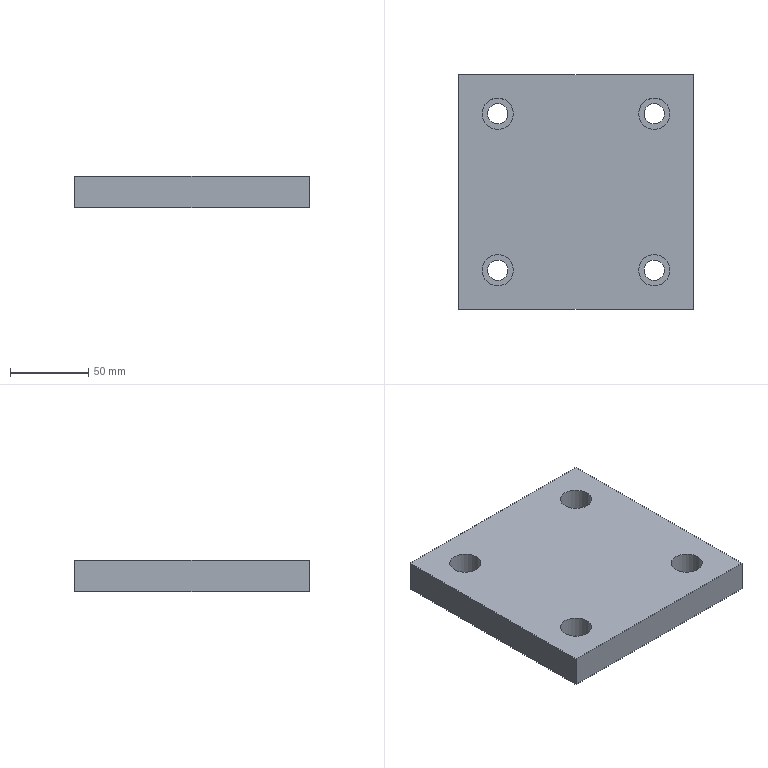Part | NX | features solid 2 | 1 solid | 18 faces | box 150 x 150 x 20 mm | volume 429222 mm3 | plane 10 | cylinder 8 | commonest cylinder face diameters 13 x4 20 x4
STEP:
#1=CARTESIAN_POINT('',(335.,1005.,-255.));
#2=VERTEX_POINT('',#1);
#3=CARTESIAN_POINT('',(335.,855.,-255.));
#4=VERTEX_POINT('',#3);
#5=CARTESIAN_POINT('',(335.,1032.5,-255.));
#6=DIRECTION('',(0.,1.,0.));
#7=VECTOR('',#6,1000.);
#8=LINE('',#5,#7);
#9=EDGE_CURVE('',#2,#4,#8,.F.);
#10=ORIENTED_EDGE('',*,*,#9,.T.);
#11=CARTESIAN_POINT('',(185.,855.,-255.));
#12=VERTEX_POINT('',#11);
#13=CARTESIAN_POINT('',(222.674,855.,-255.));
#14=DIRECTION('',(-1.,0.,0.));
#15=VECTOR('',#14,1000.);
#16=LINE('',#13,#15);
#17=EDGE_CURVE('',#12,#4,#16,.F.);
#18=ORIENTED_EDGE('',*,*,#17,.F.);
#19=CARTESIAN_POINT('',(185.,1005.,-255.));
#20=VERTEX_POINT('',#19);
#21=CARTESIAN_POINT('',(185.,1032.5,-255.));
#22=DIRECTION('',(0.,-1.,0.));
#23=VECTOR('',#22,1000.);
#24=LINE('',#21,#23);
#25=EDGE_CURVE('',#12,#20,#24,.F.);
#26=ORIENTED_EDGE('',*,*,#25,.T.);
#27=CARTESIAN_POINT('',(222.674,1005.,-255.));
#28=DIRECTION('',(-1.,0.,0.));
#29=VECTOR('',#28,1000.);
#30=LINE('',#27,#29);
#31=EDGE_CURVE('',#20,#2,#30,.F.);
#32=ORIENTED_EDGE('',*,*,#31,.T.);
#33=EDGE_LOOP('',(#10,#18,#26,#32));
#34=FACE_BOUND('',#33,.T.);
#35=CARTESIAN_POINT('',(210.,986.5,-255.));
#36=VERTEX_POINT('',#35);
#37=CARTESIAN_POINT('',(210.,980.,-255.));
#38=DIRECTION('',(0.,0.,-1.));
#39=DIRECTION('',(0.,1.,0.));
#40=AXIS2_PLACEMENT_3D('',#37,#38,#39);
#41=CIRCLE('',#40,6.5);
#42=EDGE_CURVE('',#36,#36,#41,.T.);
#43=ORIENTED_EDGE('',*,*,#42,.F.);
#44=EDGE_LOOP('',(#43));
#45=FACE_BOUND('',#44,.T.);
#46=CARTESIAN_POINT('',(310.,986.5,-255.));
#47=VERTEX_POINT('',#46);
#48=CARTESIAN_POINT('',(310.,980.,-255.));
#49=DIRECTION('',(0.,0.,-1.));
#50=DIRECTION('',(0.,1.,0.));
#51=AXIS2_PLACEMENT_3D('',#48,#49,#50);
#52=CIRCLE('',#51,6.5);
#53=EDGE_CURVE('',#47,#47,#52,.T.);
#54=ORIENTED_EDGE('',*,*,#53,.F.);
#55=EDGE_LOOP('',(#54));
#56=FACE_BOUND('',#55,.T.);
#57=CARTESIAN_POINT('',(210.,886.5,-255.));
#58=VERTEX_POINT('',#57);
#59=CARTESIAN_POINT('',(210.,880.,-255.));
#60=DIRECTION('',(0.,0.,-1.));
#61=DIRECTION('',(0.,1.,0.));
#62=AXIS2_PLACEMENT_3D('',#59,#60,#61);
#63=CIRCLE('',#62,6.5);
#64=EDGE_CURVE('',#58,#58,#63,.T.);
#65=ORIENTED_EDGE('',*,*,#64,.F.);
#66=EDGE_LOOP('',(#65));
#67=FACE_BOUND('',#66,.T.);
#68=CARTESIAN_POINT('',(310.,886.5,-255.));
#69=VERTEX_POINT('',#68);
#70=CARTESIAN_POINT('',(310.,880.,-255.));
#71=DIRECTION('',(0.,0.,-1.));
#72=DIRECTION('',(0.,1.,0.));
#73=AXIS2_PLACEMENT_3D('',#70,#71,#72);
#74=CIRCLE('',#73,6.5);
#75=EDGE_CURVE('',#69,#69,#74,.T.);
#76=ORIENTED_EDGE('',*,*,#75,.F.);
#77=EDGE_LOOP('',(#76));
#78=FACE_BOUND('',#77,.T.);
#79=CARTESIAN_POINT('',(222.674,1032.5,-255.));
#80=DIRECTION('',(0.,0.,1.));
#81=DIRECTION('',(1.,0.,0.));
#82=AXIS2_PLACEMENT_3D('',#79,#80,#81);
#83=PLANE('',#82);
#84=ADVANCED_FACE('',(#34,#45,#56,#67,#78),#83,.F.);
#85=CARTESIAN_POINT('',(185.,1005.,-235.));
#86=VERTEX_POINT('',#85);
#87=CARTESIAN_POINT('',(335.,1005.,-235.));
#88=VERTEX_POINT('',#87);
#89=CARTESIAN_POINT('',(222.674,1005.,-235.));
#90=DIRECTION('',(-1.,0.,0.));
#91=VECTOR('',#90,1000.);
#92=LINE('',#89,#91);
#93=EDGE_CURVE('',#86,#88,#92,.F.);
#94=ORIENTED_EDGE('',*,*,#93,.F.);
#95=CARTESIAN_POINT('',(185.,855.,-235.));
#96=VERTEX_POINT('',#95);
#97=CARTESIAN_POINT('',(185.,1032.5,-235.));
#98=DIRECTION('',(0.,-1.,0.));
#99=VECTOR('',#98,1000.);
#100=LINE('',#97,#99);
#101=EDGE_CURVE('',#96,#86,#100,.F.);
#102=ORIENTED_EDGE('',*,*,#101,.F.);
#103=CARTESIAN_POINT('',(335.,855.,-235.));
#104=VERTEX_POINT('',#103);
#105=CARTESIAN_POINT('',(222.674,855.,-235.));
#106=DIRECTION('',(-1.,0.,0.));
#107=VECTOR('',#106,1000.);
#108=LINE('',#105,#107);
#109=EDGE_CURVE('',#96,#104,#108,.F.);
#110=ORIENTED_EDGE('',*,*,#109,.T.);
#111=CARTESIAN_POINT('',(335.,1032.5,-235.));
#112=DIRECTION('',(0.,1.,0.));
#113=VECTOR('',#112,1000.);
#114=LINE('',#111,#113);
#115=EDGE_CURVE('',#88,#104,#114,.F.);
#116=ORIENTED_EDGE('',*,*,#115,.F.);
#117=EDGE_LOOP('',(#94,#102,#110,#116));
#118=FACE_BOUND('',#117,.T.);
#119=CARTESIAN_POINT('',(210.,990.,-235.));
#120=VERTEX_POINT('',#119);
#121=CARTESIAN_POINT('',(210.,980.,-235.));
#122=DIRECTION('',(0.,0.,-1.));
#123=DIRECTION('',(0.,1.,0.));
#124=AXIS2_PLACEMENT_3D('',#121,#122,#123);
#125=CIRCLE('',#124,10.);
#126=EDGE_CURVE('',#120,#120,#125,.T.);
#127=ORIENTED_EDGE('',*,*,#126,.T.);
#128=EDGE_LOOP('',(#127));
#129=FACE_BOUND('',#128,.T.);
#130=CARTESIAN_POINT('',(310.,990.,-235.));
#131=VERTEX_POINT('',#130);
#132=CARTESIAN_POINT('',(310.,980.,-235.));
#133=DIRECTION('',(0.,0.,-1.));
#134=DIRECTION('',(0.,1.,0.));
#135=AXIS2_PLACEMENT_3D('',#132,#133,#134);
#136=CIRCLE('',#135,10.);
#137=EDGE_CURVE('',#131,#131,#136,.T.);
#138=ORIENTED_EDGE('',*,*,#137,.T.);
#139=EDGE_LOOP('',(#138));
#140=FACE_BOUND('',#139,.T.);
#141=CARTESIAN_POINT('',(210.,890.,-235.));
#142=VERTEX_POINT('',#141);
#143=CARTESIAN_POINT('',(210.,880.,-235.));
#144=DIRECTION('',(0.,0.,-1.));
#145=DIRECTION('',(0.,1.,0.));
#146=AXIS2_PLACEMENT_3D('',#143,#144,#145);
#147=CIRCLE('',#146,10.);
#148=EDGE_CURVE('',#142,#142,#147,.T.);
#149=ORIENTED_EDGE('',*,*,#148,.T.);
#150=EDGE_LOOP('',(#149));
#151=FACE_BOUND('',#150,.T.);
#152=CARTESIAN_POINT('',(310.,890.,-235.));
#153=VERTEX_POINT('',#152);
#154=CARTESIAN_POINT('',(310.,880.,-235.));
#155=DIRECTION('',(0.,0.,-1.));
#156=DIRECTION('',(0.,1.,0.));
#157=AXIS2_PLACEMENT_3D('',#154,#155,#156);
#158=CIRCLE('',#157,10.);
#159=EDGE_CURVE('',#153,#153,#158,.T.);
#160=ORIENTED_EDGE('',*,*,#159,.T.);
#161=EDGE_LOOP('',(#160));
#162=FACE_BOUND('',#161,.T.);
#163=CARTESIAN_POINT('',(222.674,1032.5,-235.));
#164=DIRECTION('',(0.,0.,1.));
#165=DIRECTION('',(1.,0.,0.));
#166=AXIS2_PLACEMENT_3D('',#163,#164,#165);
#167=PLANE('',#166);
#168=ADVANCED_FACE('',(#118,#129,#140,#151,#162),#167,.T.);
#169=CARTESIAN_POINT('',(185.,1005.,-255.));
#170=DIRECTION('',(0.,0.,1.));
#171=VECTOR('',#170,1000.);
#172=LINE('',#169,#171);
#173=EDGE_CURVE('',#20,#86,#172,.T.);
#174=ORIENTED_EDGE('',*,*,#173,.F.);
#175=ORIENTED_EDGE('',*,*,#25,.F.);
#176=CARTESIAN_POINT('',(185.,855.,-255.));
#177=DIRECTION('',(0.,0.,1.));
#178=VECTOR('',#177,1000.);
#179=LINE('',#176,#178);
#180=EDGE_CURVE('',#12,#96,#179,.T.);
#181=ORIENTED_EDGE('',*,*,#180,.T.);
#182=ORIENTED_EDGE('',*,*,#101,.T.);
#183=EDGE_LOOP('',(#174,#175,#181,#182));
#184=FACE_BOUND('',#183,.T.);
#185=CARTESIAN_POINT('',(185.,1032.5,-255.));
#186=DIRECTION('',(1.,0.,0.));
#187=DIRECTION('',(0.,0.,1.));
#188=AXIS2_PLACEMENT_3D('',#185,#186,#187);
#189=PLANE('',#188);
#190=ADVANCED_FACE('',(#184),#189,.F.);
#191=ORIENTED_EDGE('',*,*,#115,.T.);
#192=CARTESIAN_POINT('',(335.,855.,-255.));
#193=DIRECTION('',(0.,0.,1.));
#194=VECTOR('',#193,1000.);
#195=LINE('',#192,#194);
#196=EDGE_CURVE('',#4,#104,#195,.T.);
#197=ORIENTED_EDGE('',*,*,#196,.F.);
#198=ORIENTED_EDGE('',*,*,#9,.F.);
#199=CARTESIAN_POINT('',(335.,1005.,-255.));
#200=DIRECTION('',(0.,0.,1.));
#201=VECTOR('',#200,1000.);
#202=LINE('',#199,#201);
#203=EDGE_CURVE('',#2,#88,#202,.T.);
#204=ORIENTED_EDGE('',*,*,#203,.T.);
#205=EDGE_LOOP('',(#191,#197,#198,#204));
#206=FACE_BOUND('',#205,.T.);
#207=CARTESIAN_POINT('',(335.,1007.5,-255.));
#208=DIRECTION('',(1.,0.,0.));
#209=DIRECTION('',(0.,0.,1.));
#210=AXIS2_PLACEMENT_3D('',#207,#208,#209);
#211=PLANE('',#210);
#212=ADVANCED_FACE('',(#206),#211,.T.);
#213=ORIENTED_EDGE('',*,*,#17,.T.);
#214=ORIENTED_EDGE('',*,*,#196,.T.);
#215=ORIENTED_EDGE('',*,*,#109,.F.);
#216=ORIENTED_EDGE('',*,*,#180,.F.);
#217=EDGE_LOOP('',(#213,#214,#215,#216));
#218=FACE_BOUND('',#217,.T.);
#219=CARTESIAN_POINT('',(222.674,855.,-255.));
#220=DIRECTION('',(0.,-1.,0.));
#221=DIRECTION('',(0.,0.,-1.));
#222=AXIS2_PLACEMENT_3D('',#219,#220,#221);
#223=PLANE('',#222);
#224=ADVANCED_FACE('',(#218),#223,.T.);
#225=ORIENTED_EDGE('',*,*,#75,.T.);
#226=EDGE_LOOP('',(#225));
#227=FACE_BOUND('',#226,.T.);
#228=CARTESIAN_POINT('',(310.,886.5,-249.));
#229=VERTEX_POINT('',#228);
#230=CARTESIAN_POINT('',(310.,880.,-249.));
#231=DIRECTION('',(0.,0.,-1.));
#232=DIRECTION('',(0.,1.,0.));
#233=AXIS2_PLACEMENT_3D('',#230,#231,#232);
#234=CIRCLE('',#233,6.5);
#235=EDGE_CURVE('',#229,#229,#234,.T.);
#236=ORIENTED_EDGE('',*,*,#235,.F.);
#237=EDGE_LOOP('',(#236));
#238=FACE_BOUND('',#237,.T.);
#239=CARTESIAN_POINT('',(310.,880.,-255.));
#240=DIRECTION('',(0.,0.,-1.));
#241=DIRECTION('',(0.,1.,0.));
#242=AXIS2_PLACEMENT_3D('',#239,#240,#241);
#243=CYLINDRICAL_SURFACE('',#242,6.5);
#244=ADVANCED_FACE('',(#227,#238),#243,.F.);
#245=ORIENTED_EDGE('',*,*,#235,.T.);
#246=EDGE_LOOP('',(#245));
#247=FACE_BOUND('',#246,.T.);
#248=CARTESIAN_POINT('',(310.,890.,-249.));
#249=VERTEX_POINT('',#248);
#250=CARTESIAN_POINT('',(310.,880.,-249.));
#251=DIRECTION('',(0.,0.,-1.));
#252=DIRECTION('',(0.,1.,0.));
#253=AXIS2_PLACEMENT_3D('',#250,#251,#252);
#254=CIRCLE('',#253,10.);
#255=EDGE_CURVE('',#249,#249,#254,.T.);
#256=ORIENTED_EDGE('',*,*,#255,.F.);
#257=EDGE_LOOP('',(#256));
#258=FACE_BOUND('',#257,.T.);
#259=CARTESIAN_POINT('',(310.,880.,-249.));
#260=DIRECTION('',(0.,0.,-1.));
#261=DIRECTION('',(0.,1.,0.));
#262=AXIS2_PLACEMENT_3D('',#259,#260,#261);
#263=PLANE('',#262);
#264=ADVANCED_FACE('',(#247,#258),#263,.F.);
#265=ORIENTED_EDGE('',*,*,#255,.T.);
#266=EDGE_LOOP('',(#265));
#267=FACE_BOUND('',#266,.T.);
#268=ORIENTED_EDGE('',*,*,#159,.F.);
#269=EDGE_LOOP('',(#268));
#270=FACE_BOUND('',#269,.T.);
#271=CARTESIAN_POINT('',(310.,880.,-235.));
#272=DIRECTION('',(0.,0.,-1.));
#273=DIRECTION('',(0.,1.,0.));
#274=AXIS2_PLACEMENT_3D('',#271,#272,#273);
#275=CYLINDRICAL_SURFACE('',#274,10.);
#276=ADVANCED_FACE('',(#267,#270),#275,.F.);
#277=ORIENTED_EDGE('',*,*,#64,.T.);
#278=EDGE_LOOP('',(#277));
#279=FACE_BOUND('',#278,.T.);
#280=CARTESIAN_POINT('',(210.,886.5,-249.));
#281=VERTEX_POINT('',#280);
#282=CARTESIAN_POINT('',(210.,880.,-249.));
#283=DIRECTION('',(0.,0.,-1.));
#284=DIRECTION('',(0.,1.,0.));
#285=AXIS2_PLACEMENT_3D('',#282,#283,#284);
#286=CIRCLE('',#285,6.5);
#287=EDGE_CURVE('',#281,#281,#286,.T.);
#288=ORIENTED_EDGE('',*,*,#287,.F.);
#289=EDGE_LOOP('',(#288));
#290=FACE_BOUND('',#289,.T.);
#291=CARTESIAN_POINT('',(210.,880.,-255.));
#292=DIRECTION('',(0.,0.,-1.));
#293=DIRECTION('',(0.,1.,0.));
#294=AXIS2_PLACEMENT_3D('',#291,#292,#293);
#295=CYLINDRICAL_SURFACE('',#294,6.5);
#296=ADVANCED_FACE('',(#279,#290),#295,.F.);
#297=ORIENTED_EDGE('',*,*,#287,.T.);
#298=EDGE_LOOP('',(#297));
#299=FACE_BOUND('',#298,.T.);
#300=CARTESIAN_POINT('',(210.,890.,-249.));
#301=VERTEX_POINT('',#300);
#302=CARTESIAN_POINT('',(210.,880.,-249.));
#303=DIRECTION('',(0.,0.,-1.));
#304=DIRECTION('',(0.,1.,0.));
#305=AXIS2_PLACEMENT_3D('',#302,#303,#304);
#306=CIRCLE('',#305,10.);
#307=EDGE_CURVE('',#301,#301,#306,.T.);
#308=ORIENTED_EDGE('',*,*,#307,.F.);
#309=EDGE_LOOP('',(#308));
#310=FACE_BOUND('',#309,.T.);
#311=CARTESIAN_POINT('',(210.,880.,-249.));
#312=DIRECTION('',(0.,0.,-1.));
#313=DIRECTION('',(0.,1.,0.));
#314=AXIS2_PLACEMENT_3D('',#311,#312,#313);
#315=PLANE('',#314);
#316=ADVANCED_FACE('',(#299,#310),#315,.F.);
#317=ORIENTED_EDGE('',*,*,#307,.T.);
#318=EDGE_LOOP('',(#317));
#319=FACE_BOUND('',#318,.T.);
#320=ORIENTED_EDGE('',*,*,#148,.F.);
#321=EDGE_LOOP('',(#320));
#322=FACE_BOUND('',#321,.T.);
#323=CARTESIAN_POINT('',(210.,880.,-235.));
#324=DIRECTION('',(0.,0.,-1.));
#325=DIRECTION('',(0.,1.,0.));
#326=AXIS2_PLACEMENT_3D('',#323,#324,#325);
#327=CYLINDRICAL_SURFACE('',#326,10.);
#328=ADVANCED_FACE('',(#319,#322),#327,.F.);
#329=CARTESIAN_POINT('',(310.,986.5,-249.));
#330=VERTEX_POINT('',#329);
#331=CARTESIAN_POINT('',(310.,980.,-249.));
#332=DIRECTION('',(0.,0.,-1.));
#333=DIRECTION('',(0.,1.,0.));
#334=AXIS2_PLACEMENT_3D('',#331,#332,#333);
#335=CIRCLE('',#334,6.5);
#336=EDGE_CURVE('',#330,#330,#335,.T.);
#337=ORIENTED_EDGE('',*,*,#336,.T.);
#338=EDGE_LOOP('',(#337));
#339=FACE_BOUND('',#338,.T.);
#340=CARTESIAN_POINT('',(310.,990.,-249.));
#341=VERTEX_POINT('',#340);
#342=CARTESIAN_POINT('',(310.,980.,-249.));
#343=DIRECTION('',(0.,0.,-1.));
#344=DIRECTION('',(0.,1.,0.));
#345=AXIS2_PLACEMENT_3D('',#342,#343,#344);
#346=CIRCLE('',#345,10.);
#347=EDGE_CURVE('',#341,#341,#346,.T.);
#348=ORIENTED_EDGE('',*,*,#347,.F.);
#349=EDGE_LOOP('',(#348));
#350=FACE_BOUND('',#349,.T.);
#351=CARTESIAN_POINT('',(310.,980.,-249.));
#352=DIRECTION('',(0.,0.,-1.));
#353=DIRECTION('',(0.,1.,0.));
#354=AXIS2_PLACEMENT_3D('',#351,#352,#353);
#355=PLANE('',#354);
#356=ADVANCED_FACE('',(#339,#350),#355,.F.);
#357=CARTESIAN_POINT('',(210.,986.5,-249.));
#358=VERTEX_POINT('',#357);
#359=CARTESIAN_POINT('',(210.,980.,-249.));
#360=DIRECTION('',(0.,0.,-1.));
#361=DIRECTION('',(0.,1.,0.));
#362=AXIS2_PLACEMENT_3D('',#359,#360,#361);
#363=CIRCLE('',#362,6.5);
#364=EDGE_CURVE('',#358,#358,#363,.T.);
#365=ORIENTED_EDGE('',*,*,#364,.T.);
#366=EDGE_LOOP('',(#365));
#367=FACE_BOUND('',#366,.T.);
#368=CARTESIAN_POINT('',(210.,990.,-249.));
#369=VERTEX_POINT('',#368);
#370=CARTESIAN_POINT('',(210.,980.,-249.));
#371=DIRECTION('',(0.,0.,-1.));
#372=DIRECTION('',(0.,1.,0.));
#373=AXIS2_PLACEMENT_3D('',#370,#371,#372);
#374=CIRCLE('',#373,10.);
#375=EDGE_CURVE('',#369,#369,#374,.T.);
#376=ORIENTED_EDGE('',*,*,#375,.F.);
#377=EDGE_LOOP('',(#376));
#378=FACE_BOUND('',#377,.T.);
#379=CARTESIAN_POINT('',(210.,980.,-249.));
#380=DIRECTION('',(0.,0.,-1.));
#381=DIRECTION('',(0.,1.,0.));
#382=AXIS2_PLACEMENT_3D('',#379,#380,#381);
#383=PLANE('',#382);
#384=ADVANCED_FACE('',(#367,#378),#383,.F.);
#385=ORIENTED_EDGE('',*,*,#53,.T.);
#386=EDGE_LOOP('',(#385));
#387=FACE_BOUND('',#386,.T.);
#388=ORIENTED_EDGE('',*,*,#336,.F.);
#389=EDGE_LOOP('',(#388));
#390=FACE_BOUND('',#389,.T.);
#391=CARTESIAN_POINT('',(310.,980.,-255.));
#392=DIRECTION('',(0.,0.,-1.));
#393=DIRECTION('',(0.,1.,0.));
#394=AXIS2_PLACEMENT_3D('',#391,#392,#393);
#395=CYLINDRICAL_SURFACE('',#394,6.5);
#396=ADVANCED_FACE('',(#387,#390),#395,.F.);
#397=ORIENTED_EDGE('',*,*,#42,.T.);
#398=EDGE_LOOP('',(#397));
#399=FACE_BOUND('',#398,.T.);
#400=ORIENTED_EDGE('',*,*,#364,.F.);
#401=EDGE_LOOP('',(#400));
#402=FACE_BOUND('',#401,.T.);
#403=CARTESIAN_POINT('',(210.,980.,-255.));
#404=DIRECTION('',(0.,0.,-1.));
#405=DIRECTION('',(0.,1.,0.));
#406=AXIS2_PLACEMENT_3D('',#403,#404,#405);
#407=CYLINDRICAL_SURFACE('',#406,6.5);
#408=ADVANCED_FACE('',(#399,#402),#407,.F.);
#409=ORIENTED_EDGE('',*,*,#347,.T.);
#410=EDGE_LOOP('',(#409));
#411=FACE_BOUND('',#410,.T.);
#412=ORIENTED_EDGE('',*,*,#137,.F.);
#413=EDGE_LOOP('',(#412));
#414=FACE_BOUND('',#413,.T.);
#415=CARTESIAN_POINT('',(310.,980.,-235.));
#416=DIRECTION('',(0.,0.,-1.));
#417=DIRECTION('',(0.,1.,0.));
#418=AXIS2_PLACEMENT_3D('',#415,#416,#417);
#419=CYLINDRICAL_SURFACE('',#418,10.);
#420=ADVANCED_FACE('',(#411,#414),#419,.F.);
#421=ORIENTED_EDGE('',*,*,#375,.T.);
#422=EDGE_LOOP('',(#421));
#423=FACE_BOUND('',#422,.T.);
#424=ORIENTED_EDGE('',*,*,#126,.F.);
#425=EDGE_LOOP('',(#424));
#426=FACE_BOUND('',#425,.T.);
#427=CARTESIAN_POINT('',(210.,980.,-235.));
#428=DIRECTION('',(0.,0.,-1.));
#429=DIRECTION('',(0.,1.,0.));
#430=AXIS2_PLACEMENT_3D('',#427,#428,#429);
#431=CYLINDRICAL_SURFACE('',#430,10.);
#432=ADVANCED_FACE('',(#423,#426),#431,.F.);
#433=ORIENTED_EDGE('',*,*,#203,.F.);
#434=ORIENTED_EDGE('',*,*,#31,.F.);
#435=ORIENTED_EDGE('',*,*,#173,.T.);
#436=ORIENTED_EDGE('',*,*,#93,.T.);
#437=EDGE_LOOP('',(#433,#434,#435,#436));
#438=FACE_BOUND('',#437,.T.);
#439=CARTESIAN_POINT('',(222.674,1005.,-255.));
#440=DIRECTION('',(0.,-1.,0.));
#441=DIRECTION('',(0.,0.,-1.));
#442=AXIS2_PLACEMENT_3D('',#439,#440,#441);
#443=PLANE('',#442);
#444=ADVANCED_FACE('',(#438),#443,.F.);
#445=CLOSED_SHELL('',(#84,#168,#190,#212,#224,#244,#264,#276,#296,#316,#328,#356,#384,#396,#408,#420,#432,#444));
#446=MANIFOLD_SOLID_BREP('',#445);
#447=(LENGTH_UNIT()NAMED_UNIT(*)SI_UNIT(.MILLI.,.METRE.));
#448=UNCERTAINTY_MEASURE_WITH_UNIT(LENGTH_MEASURE(0.00001),#447,'','');
#449=(NAMED_UNIT(*)PLANE_ANGLE_UNIT()SI_UNIT($,.RADIAN.));
#450=(NAMED_UNIT(*)SI_UNIT($,.STERADIAN.)SOLID_ANGLE_UNIT());
#451=(GEOMETRIC_REPRESENTATION_CONTEXT(3)GLOBAL_UNCERTAINTY_ASSIGNED_CONTEXT((#448))GLOBAL_UNIT_ASSIGNED_CONTEXT((#447,#449,#450))REPRESENTATION_CONTEXT('',''));
#452=ADVANCED_BREP_SHAPE_REPRESENTATION('',(#446),#451);